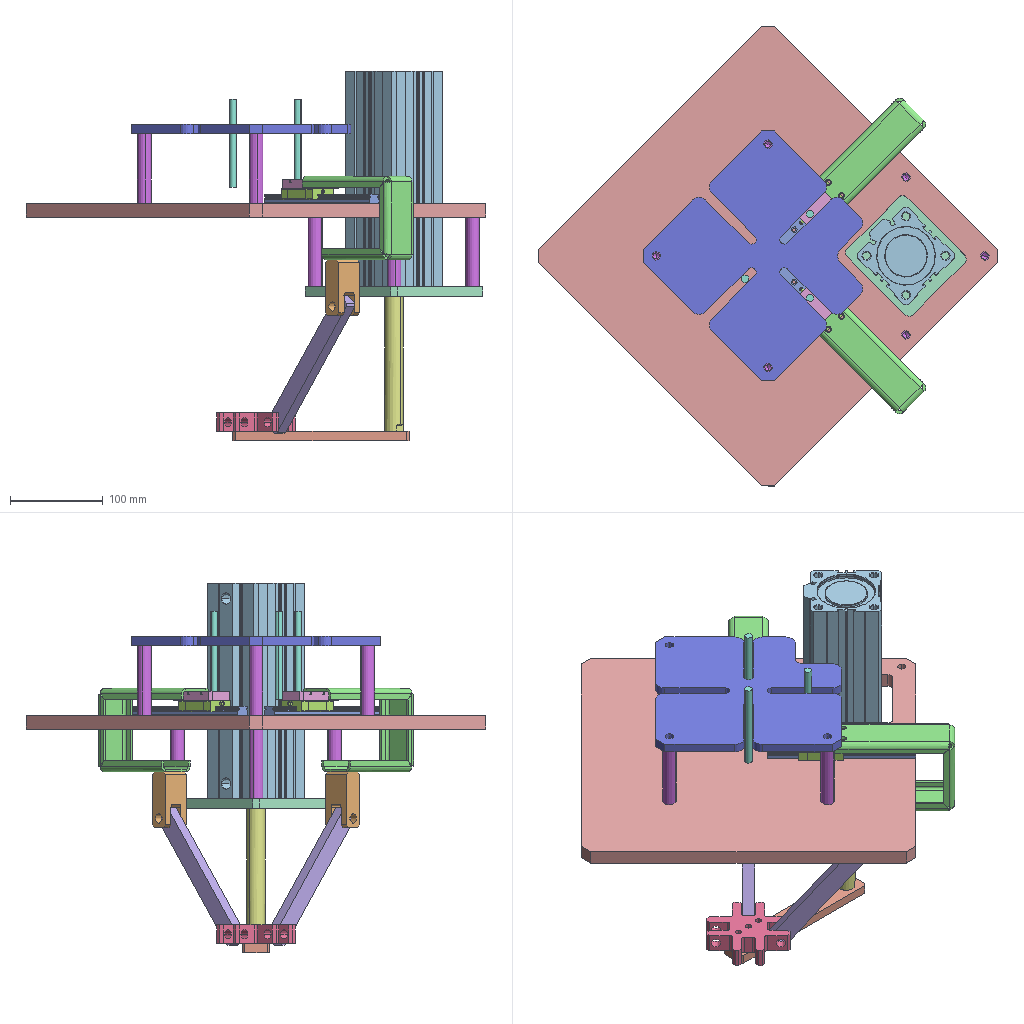Assembly | SolidWorks | 15 different items | 29 placed | box 495 x 495 x 398 mm
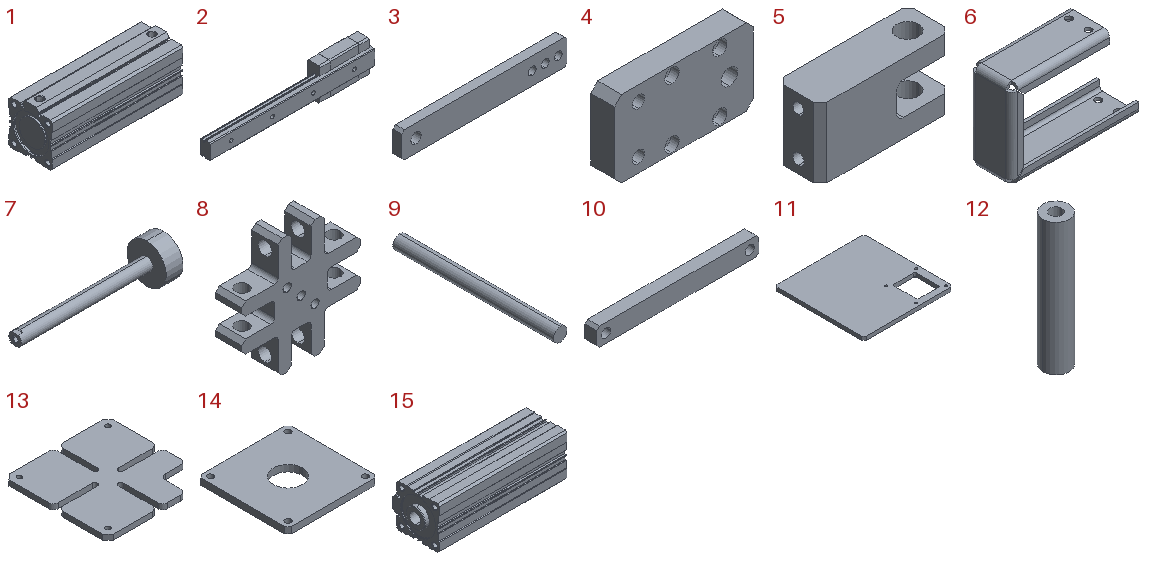Parts list (item | name | quantity | parent item | size | volume | features):
1 | (subassembly) | x1 | - | 250 x 77 x 84 mm | 780379 mm3 | -
2 | (subassembly) | x2 | - | 160 x 16 x 32 mm | 35249 mm3 | -
3 | - | x1 | - | 190 x 10 x 30 mm | 53781 mm3 | features HoleWzd 2, Chamfer 1, Extrusion 1
4 | - | x2 | - | 58 x 10 x 32 mm | 17000 mm3 | features HoleWzd 3, Chamfer 1, Extrusion 1
5 | - | x2 | - | 60 x 20 x 32 mm | 28592 mm3 | features ICE 2, Chamfer 1, Extrusion 1, Fillet 1, HoleWzd 1
6 | - | x2 | - | 130 x 43 x 90 mm | 51061 mm3 | features EdgeFlange 3, HoleWzd 2, MirrorPattern 2, FlatPattern 1, ICE 1, SMBaseFlange 1, SheetMetal 1
7 | - | x1 | in 1 | 236.5 x 62.5 x 62.5 mm | 147452 mm3 | features BaseBody 1
8 | - | x1 | - | 90 x 20 x 90 mm | 62065 mm3 | features Chamfer 4, CirPattern 3, ICE 3, Fillet 2, HoleWzd 2, Extrusion 1
9 | - | x3 | - | 8 x 95 x 8 mm | 4775 mm3 | features Extrusion 1
10 | - | x2 | - | 177.8 x 13 x 20 mm | 43952 mm3 | features Chamfer 1, Extrusion 1, ICE 1, LPattern 1
11 | - | x1 | - | 360 x 360 x 15 mm | 1802505 mm3 | features Chamfer 1, Extrusion 1, Fillet 1, HoleWzd 1, ICE 1
12 | - | x8 | - | 15 x 15 x 75 mm | 11770 mm3 | features HoleWzd 2, Extrusion 1
13 | - | x1 | - | 200 x 200 x 10 mm | 338089 mm3 | features ICE 3, CirPattern 2, Fillet 2, Chamfer 1, DelFace 1, Extrusion 1, HoleWzd 1
14 | - | x1 | - | 140 x 140 x 10 mm | 177051 mm3 | features Chamfer 1, Extrusion 1, HoleWzd 1, ICE 1, LPattern 1
15 | - | x1 | in 1 | 237 x 84 x 77 mm | 632926 mm3 | features BaseBody 1
Mates (type | each side: item.copy, entity, surface, feature):
In the top assembly
Concentric | 4.1 face cylinder M8 Tapped Hole1 | 9.1 face cylinder Boss-Extrude1
Concentric | 4.2 face cylinder M8 Tapped Hole1 | 9.2 face cylinder Boss-Extrude1
Coincident | 9.3 face plane Boss-Extrude1 | 9.2 face plane Boss-Extrude1
Coincident | 4.1 face plane Boss-Extrude1 | 6.1 face plane Base-Flange1
Concentric | 4.1 face cylinder M6 Tapped Hole1 | 6.1 face cylinder Ø6.5 (6.5) Diameter Hole2 | 2 times
Concentric | 4.2 face cylinder M6 Tapped Hole1 | 6.2 face cylinder Ø6.5 (6.5) Diameter Hole2 | 2 times
Coincident | 4.2 face plane Boss-Extrude1 | 6.2 face plane Base-Flange1
Concentric | 5.1 face cylinder M6 Tapped Hole1 | 6.2 face cylinder Ø6.5 (6.5) Diameter Hole1 | 2 times
Coincident | 5.1 face plane Boss-Extrude1 | 6.2 face plane Edge-Flange2
Width | 5.1 face plane Boss-Extrude1 | 5.1 face plane Boss-Extrude1 | 10.1 face plane Boss-Extrude1 | 10.1 face plane Boss-Extrude1
Concentric | 5.1 face cylinder Cut-Extrude1 | 10.1 face cylinder LPattern1
Concentric | 5.2 face cylinder M6 Tapped Hole1 | 6.1 face cylinder Ø6.5 (6.5) Diameter Hole1 | 2 times
Coincident | 5.2 face plane Boss-Extrude1 | 6.1 face plane Edge-Flange2
Width | 5.2 face plane Boss-Extrude1 | 5.2 face plane Boss-Extrude1 | 10.2 face plane Boss-Extrude1 | 10.2 face plane Boss-Extrude1
Concentric | 5.2 face cylinder Cut-Extrude1 | 10.2 face cylinder LPattern1
Parallel | 11.1 face plane Boss-Extrude1 | 8.1 face plane Boss-Extrude1
Concentric | 10.1 face cylinder Cut-Extrude1 | 8.1 face cylinder CirPattern4
Concentric | 10.2 face cylinder Cut-Extrude1 | 8.1 face cylinder Cut-Extrude3
Width | 8.1 face plane CirPattern2 | 8.1 face plane CirPattern2 | 10.1 face plane Boss-Extrude1 | 10.1 face plane Boss-Extrude1
Width | 8.1 face plane CirPattern3 | 8.1 face plane Cut-Extrude2 | 10.2 face plane Boss-Extrude1 | 10.2 face plane Boss-Extrude1
Coincident | 15.1 face plane Input1 | 14.1 face plane Boss-Extrude1
Width | 14.1 face plane Boss-Extrude1 | 14.1 face plane Boss-Extrude1 | 15.1 face plane Input1 | 15.1 face plane Input1 | 2 times
Concentric | 12.1 face cylinder M8 Tapped Hole1 | 14.1 face cylinder LPattern1
Coincident | 12.1 face plane Boss-Extrude1 | 14.1 face plane Boss-Extrude1
Coincident | 14.1 face plane Boss-Extrude1 | 12.2 face plane Boss-Extrude1
Concentric | 14.1 face cylinder LPattern1 | 12.2 face cylinder M8 Tapped Hole1
Concentric | 14.1 face cylinder Ø9.0 (9) Diameter Hole1 | 12.3 face cylinder M8 Tapped Hole1
Coincident | 14.1 face plane Boss-Extrude1 | 12.3 face plane Boss-Extrude1
Concentric | 14.1 face cylinder LPattern1 | 12.4 face cylinder M8 Tapped Hole2
Coincident | 14.1 face plane Boss-Extrude1 | 12.4 face plane Boss-Extrude1
Coincident | 11.1 face plane Boss-Extrude1 | 12.3 face plane Boss-Extrude1
Concentric | 11.1 face cylinder Ø9.0 (9) Diameter Hole1 | 12.3 face cylinder M8 Tapped Hole2
Concentric | 11.1 face cylinder Ø9.0 (9) Diameter Hole1 | 12.1 face cylinder M8 Tapped Hole2
Concentric | 8.1 face cylinder M8 Tapped Hole2 | 3.1 face cylinder Ø9.0 (9) Diameter Hole1 | 2 times
Concentric | 8.1 face cylinder M8 Tapped Hole1 | 3.1 face cylinder Ø9.0 (9) Diameter Hole1
Coincident | 8.1 face plane Boss-Extrude1 | 3.1 face plane Boss-Extrude1
Coincident | 7.1 face plane Input1 | 3.1 face plane Boss-Extrude1
Coincident | 11.1 face plane Boss-Extrude1 | 12.5 face plane Boss-Extrude1 | 2 times
Coincident | 12.5 face plane Boss-Extrude1 | 13.1 face plane Boss-Extrude1
Concentric | 12.5 face cylinder M8 Tapped Hole2 | 13.1 face cylinder Ø9.0 (9) Diameter Hole1
Width | 11.1 face plane Boss-Extrude1 | 11.1 face plane Boss-Extrude1 | 13.1 face plane Boss-Extrude1 | 13.1 face plane Boss-Extrude1 | 2 times
Concentric | 13.1 face cylinder CirPattern1 | 12.6 face cylinder Boss-Extrude1
Coincident | 13.1 face plane Boss-Extrude1 | 12.6 face plane Boss-Extrude1
In subassembly 1
LimitDistanceDim | 7.2 face plane Input1 | 15.2 face plane Input1
Concentric | 15.2 face cylinder Input1 | 7.2 face cylinder Input1
Parallel | 15.2 face plane Input1 | 7.2 face plane Input1